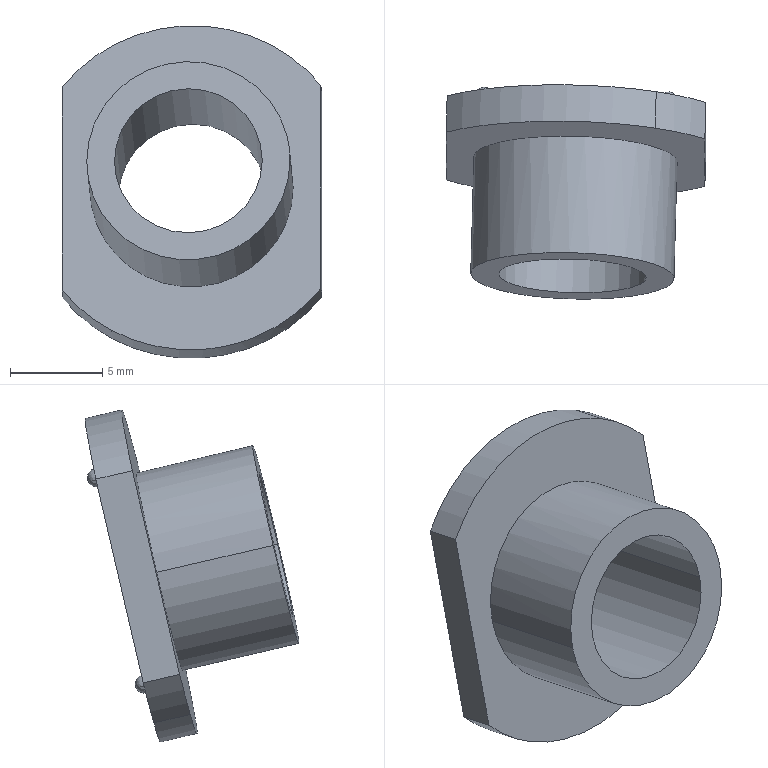Part | STEP file | FNA6101013 | 1 solid | 17 faces | box 14.049 x 11.577 x 17.992 mm | volume 641.835 mm3 | cylinder 8 | plane 5 | sphere 4 | commonest cylinder face diameters 18 x4 8 x2 11 x2
STEP:
#1=CARTESIAN_POINT('',(1542.752,-683.145,923.779));
#2=VERTEX_POINT('',#1);
#3=CARTESIAN_POINT('',(1542.752,-682.919,924.753));
#4=VERTEX_POINT('',#3);
#5=CARTESIAN_POINT('',(1542.752,-683.145,923.779));
#6=CARTESIAN_POINT('',(1542.624,-683.142,923.778));
#7=CARTESIAN_POINT('',(1542.496,-683.129,923.818));
#8=CARTESIAN_POINT('',(1542.386,-683.108,923.897));
#9=CARTESIAN_POINT('',(1542.2,-683.041,924.161));
#10=CARTESIAN_POINT('',(1542.249,-682.965,924.495));
#11=CARTESIAN_POINT('',(1542.38,-682.929,924.667));
#12=CARTESIAN_POINT('',(1542.566,-682.914,924.752));
#13=CARTESIAN_POINT('',(1542.752,-682.919,924.753));
#14=B_SPLINE_CURVE_WITH_KNOTS('',5,(#5,#6,#7,#8,#9,#10,#11,#12,#13),.UNSPECIFIED.,.F.,.U.,(6,3,6),(0.,0.9047,2.221),.UNSPECIFIED.);
#15=EDGE_CURVE('',#2,#4,#14,.T.);
#16=ORIENTED_EDGE('',*,*,#15,.T.);
#17=CARTESIAN_POINT('',(1542.752,-683.145,923.779));
#18=CARTESIAN_POINT('',(1542.88,-683.148,923.78));
#19=CARTESIAN_POINT('',(1543.008,-683.142,923.821));
#20=CARTESIAN_POINT('',(1543.118,-683.126,923.901));
#21=CARTESIAN_POINT('',(1543.305,-683.07,924.167));
#22=CARTESIAN_POINT('',(1543.255,-682.991,924.501));
#23=CARTESIAN_POINT('',(1543.124,-682.948,924.671));
#24=CARTESIAN_POINT('',(1542.938,-682.924,924.754));
#25=CARTESIAN_POINT('',(1542.752,-682.919,924.753));
#26=B_SPLINE_CURVE_WITH_KNOTS('',5,(#17,#18,#19,#20,#21,#22,#23,#24,#25),.UNSPECIFIED.,.F.,.U.,(6,3,6),(0.,0.9047,2.221),.UNSPECIFIED.);
#27=EDGE_CURVE('',#4,#2,#26,.F.);
#28=ORIENTED_EDGE('',*,*,#27,.T.);
#29=EDGE_LOOP('',(#16,#28));
#30=FACE_OUTER_BOUND('',#29,.T.);
#31=CARTESIAN_POINT('',(1542.752,-683.032,924.266));
#32=DIRECTION('',(0.,0.2262,0.9741));
#33=DIRECTION('',(0.9997,-0.02569,0.005964));
#34=AXIS2_PLACEMENT_3D('',#31,#32,#33);
#35=SPHERICAL_SURFACE('',#34,0.5);
#36=ADVANCED_FACE('',(#30),#35,.T.);
#37=CARTESIAN_POINT('',(1530.756,-682.739,924.127));
#38=VERTEX_POINT('',#37);
#39=CARTESIAN_POINT('',(1542.067,-682.523,926.378));
#40=VERTEX_POINT('',#39);
#41=CARTESIAN_POINT('',(1537.754,-684.198,918.659));
#42=DIRECTION('',(0.02637,0.9738,-0.2261));
#43=AXIS2_PLACEMENT_3D('',#41,#42,$);
#44=CIRCLE('',#43,9.);
#45=EDGE_CURVE('',#38,#40,#44,.T.);
#46=ORIENTED_EDGE('',*,*,#45,.T.);
#47=CARTESIAN_POINT('',(1544.751,-683.099,924.211));
#48=VERTEX_POINT('',#47);
#49=CARTESIAN_POINT('',(1537.754,-684.198,918.659));
#50=DIRECTION('',(0.02637,0.9738,-0.2261));
#51=AXIS2_PLACEMENT_3D('',#49,#50,$);
#52=CIRCLE('',#51,9.);
#53=EDGE_CURVE('',#40,#48,#52,.T.);
#54=ORIENTED_EDGE('',*,*,#53,.T.);
#55=CARTESIAN_POINT('',(1544.751,-685.658,913.19));
#56=VERTEX_POINT('',#55);
#57=CARTESIAN_POINT('',(1544.751,-684.378,918.701));
#58=DIRECTION('',(0.,-0.2262,-0.9741));
#59=VECTOR('',#58,1.);
#60=LINE('',#57,#59);
#61=EDGE_CURVE('',#48,#56,#60,.T.);
#62=ORIENTED_EDGE('',*,*,#61,.T.);
#63=CARTESIAN_POINT('',(1533.441,-685.874,910.939));
#64=VERTEX_POINT('',#63);
#65=CARTESIAN_POINT('',(1537.754,-684.198,918.659));
#66=DIRECTION('',(0.02637,0.9738,-0.2261));
#67=AXIS2_PLACEMENT_3D('',#65,#66,$);
#68=CIRCLE('',#67,9.);
#69=EDGE_CURVE('',#56,#64,#68,.T.);
#70=ORIENTED_EDGE('',*,*,#69,.T.);
#71=CARTESIAN_POINT('',(1530.756,-685.298,913.107));
#72=VERTEX_POINT('',#71);
#73=CARTESIAN_POINT('',(1537.754,-684.198,918.659));
#74=DIRECTION('',(0.02637,0.9738,-0.2261));
#75=AXIS2_PLACEMENT_3D('',#73,#74,$);
#76=CIRCLE('',#75,9.);
#77=EDGE_CURVE('',#64,#72,#76,.T.);
#78=ORIENTED_EDGE('',*,*,#77,.T.);
#79=CARTESIAN_POINT('',(1530.756,-684.019,918.617));
#80=DIRECTION('',(0.,0.2262,0.9741));
#81=VECTOR('',#80,1.);
#82=LINE('',#79,#81);
#83=EDGE_CURVE('',#72,#38,#82,.T.);
#84=ORIENTED_EDGE('',*,*,#83,.T.);
#85=EDGE_LOOP('',(#46,#54,#62,#70,#78,#84));
#86=FACE_OUTER_BOUND('',#85,.T.);
#87=CARTESIAN_POINT('',(1532.756,-682.888,923.72));
#88=VERTEX_POINT('',#87);
#89=CARTESIAN_POINT('',(1532.756,-682.662,924.694));
#90=VERTEX_POINT('',#89);
#91=CARTESIAN_POINT('',(1532.756,-682.888,923.72));
#92=CARTESIAN_POINT('',(1532.692,-682.886,923.719));
#93=CARTESIAN_POINT('',(1532.628,-682.882,923.729));
#94=CARTESIAN_POINT('',(1532.567,-682.876,923.748));
#95=CARTESIAN_POINT('',(1532.452,-682.86,923.806));
#96=CARTESIAN_POINT('',(1532.361,-682.837,923.895));
#97=CARTESIAN_POINT('',(1532.324,-682.823,923.947));
#98=CARTESIAN_POINT('',(1532.267,-682.796,924.061));
#99=CARTESIAN_POINT('',(1532.25,-682.766,924.186));
#100=CARTESIAN_POINT('',(1532.252,-682.751,924.25));
#101=CARTESIAN_POINT('',(1532.276,-682.723,924.374));
#102=CARTESIAN_POINT('',(1532.34,-682.699,924.485));
#103=CARTESIAN_POINT('',(1532.381,-682.688,924.535));
#104=CARTESIAN_POINT('',(1532.472,-682.672,924.617));
#105=CARTESIAN_POINT('',(1532.584,-682.663,924.668));
#106=CARTESIAN_POINT('',(1532.64,-682.661,924.685));
#107=CARTESIAN_POINT('',(1532.698,-682.66,924.693));
#108=CARTESIAN_POINT('',(1532.756,-682.662,924.694));
#109=B_SPLINE_CURVE_WITH_KNOTS('',5,(#91,#92,#93,#94,#95,#96,#97,#98,#99,#100,#101,#102,#103,#104,#105,#106,#107,#108),.UNSPECIFIED.,.F.,.U.,(6,3,3,3,3,6),(0.,0.4508,0.9047,1.358,1.812,2.221),.UNSPECIFIED.);
#110=EDGE_CURVE('',#88,#90,#109,.T.);
#111=ORIENTED_EDGE('',*,*,#110,.F.);
#112=CARTESIAN_POINT('',(1532.756,-682.888,923.72));
#113=CARTESIAN_POINT('',(1532.819,-682.89,923.72));
#114=CARTESIAN_POINT('',(1532.883,-682.889,923.73));
#115=CARTESIAN_POINT('',(1532.945,-682.886,923.75));
#116=CARTESIAN_POINT('',(1533.06,-682.875,923.809));
#117=CARTESIAN_POINT('',(1533.15,-682.857,923.9));
#118=CARTESIAN_POINT('',(1533.188,-682.846,923.952));
#119=CARTESIAN_POINT('',(1533.244,-682.821,924.067));
#120=CARTESIAN_POINT('',(1533.261,-682.792,924.192));
#121=CARTESIAN_POINT('',(1533.259,-682.777,924.256));
#122=CARTESIAN_POINT('',(1533.235,-682.748,924.38));
#123=CARTESIAN_POINT('',(1533.171,-682.72,924.49));
#124=CARTESIAN_POINT('',(1533.131,-682.708,924.54));
#125=CARTESIAN_POINT('',(1533.039,-682.687,924.62));
#126=CARTESIAN_POINT('',(1532.928,-682.672,924.67));
#127=CARTESIAN_POINT('',(1532.871,-682.667,924.686));
#128=CARTESIAN_POINT('',(1532.813,-682.663,924.694));
#129=CARTESIAN_POINT('',(1532.756,-682.662,924.694));
#130=B_SPLINE_CURVE_WITH_KNOTS('',5,(#112,#113,#114,#115,#116,#117,#118,#119,#120,#121,#122,#123,#124,#125,#126,#127,#128,#129),.UNSPECIFIED.,.F.,.U.,(6,3,3,3,3,6),(0.,0.4508,0.9047,1.358,1.812,2.221),.UNSPECIFIED.);
#131=EDGE_CURVE('',#90,#88,#130,.F.);
#132=ORIENTED_EDGE('',*,*,#131,.F.);
#133=EDGE_LOOP('',(#111,#132));
#134=FACE_BOUND('',#133,.T.);
#135=ORIENTED_EDGE('',*,*,#15,.F.);
#136=ORIENTED_EDGE('',*,*,#27,.F.);
#137=EDGE_LOOP('',(#135,#136));
#138=FACE_BOUND('',#137,.T.);
#139=CARTESIAN_POINT('',(1542.752,-685.509,913.598));
#140=VERTEX_POINT('',#139);
#141=CARTESIAN_POINT('',(1542.752,-685.735,912.624));
#142=VERTEX_POINT('',#141);
#143=CARTESIAN_POINT('',(1542.752,-685.735,912.624));
#144=CARTESIAN_POINT('',(1542.688,-685.733,912.624));
#145=CARTESIAN_POINT('',(1542.625,-685.729,912.633));
#146=CARTESIAN_POINT('',(1542.563,-685.723,912.653));
#147=CARTESIAN_POINT('',(1542.448,-685.707,912.71));
#148=CARTESIAN_POINT('',(1542.358,-685.683,912.8));
#149=CARTESIAN_POINT('',(1542.32,-685.67,912.852));
#150=CARTESIAN_POINT('',(1542.264,-685.642,912.965));
#151=CARTESIAN_POINT('',(1542.246,-685.613,913.091));
#152=CARTESIAN_POINT('',(1542.248,-685.598,913.154));
#153=CARTESIAN_POINT('',(1542.273,-685.57,913.279));
#154=CARTESIAN_POINT('',(1542.336,-685.546,913.39));
#155=CARTESIAN_POINT('',(1542.377,-685.535,913.44));
#156=CARTESIAN_POINT('',(1542.468,-685.519,913.521));
#157=CARTESIAN_POINT('',(1542.58,-685.51,913.573));
#158=CARTESIAN_POINT('',(1542.636,-685.508,913.589));
#159=CARTESIAN_POINT('',(1542.694,-685.507,913.598));
#160=CARTESIAN_POINT('',(1542.752,-685.509,913.598));
#161=B_SPLINE_CURVE_WITH_KNOTS('',5,(#143,#144,#145,#146,#147,#148,#149,#150,#151,#152,#153,#154,#155,#156,#157,#158,#159,#160),.UNSPECIFIED.,.F.,.U.,(6,3,3,3,3,6),(0.,0.4508,0.9047,1.358,1.812,2.221),.UNSPECIFIED.);
#162=EDGE_CURVE('',#140,#142,#161,.F.);
#163=ORIENTED_EDGE('',*,*,#162,.T.);
#164=CARTESIAN_POINT('',(1542.752,-685.735,912.624));
#165=CARTESIAN_POINT('',(1542.816,-685.737,912.624));
#166=CARTESIAN_POINT('',(1542.88,-685.736,912.635));
#167=CARTESIAN_POINT('',(1542.941,-685.733,912.655));
#168=CARTESIAN_POINT('',(1543.056,-685.722,912.714));
#169=CARTESIAN_POINT('',(1543.147,-685.704,912.805));
#170=CARTESIAN_POINT('',(1543.184,-685.693,912.857));
#171=CARTESIAN_POINT('',(1543.241,-685.668,912.971));
#172=CARTESIAN_POINT('',(1543.258,-685.639,913.097));
#173=CARTESIAN_POINT('',(1543.256,-685.624,913.16));
#174=CARTESIAN_POINT('',(1543.231,-685.595,913.285));
#175=CARTESIAN_POINT('',(1543.168,-685.567,913.395));
#176=CARTESIAN_POINT('',(1543.127,-685.555,913.444));
#177=CARTESIAN_POINT('',(1543.036,-685.533,913.525));
#178=CARTESIAN_POINT('',(1542.924,-685.519,913.575));
#179=CARTESIAN_POINT('',(1542.868,-685.514,913.591));
#180=CARTESIAN_POINT('',(1542.81,-685.51,913.598));
#181=CARTESIAN_POINT('',(1542.752,-685.509,913.598));
#182=B_SPLINE_CURVE_WITH_KNOTS('',5,(#164,#165,#166,#167,#168,#169,#170,#171,#172,#173,#174,#175,#176,#177,#178,#179,#180,#181),.UNSPECIFIED.,.F.,.U.,(6,3,3,3,3,6),(0.,0.4508,0.9047,1.358,1.812,2.221),.UNSPECIFIED.);
#183=EDGE_CURVE('',#142,#140,#182,.T.);
#184=ORIENTED_EDGE('',*,*,#183,.T.);
#185=EDGE_LOOP('',(#163,#184));
#186=FACE_BOUND('',#185,.T.);
#187=CARTESIAN_POINT('',(1532.756,-685.252,913.538));
#188=VERTEX_POINT('',#187);
#189=CARTESIAN_POINT('',(1532.756,-685.478,912.564));
#190=VERTEX_POINT('',#189);
#191=CARTESIAN_POINT('',(1532.756,-685.478,912.564));
#192=CARTESIAN_POINT('',(1532.692,-685.476,912.564));
#193=CARTESIAN_POINT('',(1532.628,-685.472,912.573));
#194=CARTESIAN_POINT('',(1532.567,-685.466,912.593));
#195=CARTESIAN_POINT('',(1532.452,-685.45,912.65));
#196=CARTESIAN_POINT('',(1532.361,-685.427,912.74));
#197=CARTESIAN_POINT('',(1532.324,-685.413,912.792));
#198=CARTESIAN_POINT('',(1532.267,-685.386,912.906));
#199=CARTESIAN_POINT('',(1532.25,-685.356,913.031));
#200=CARTESIAN_POINT('',(1532.252,-685.341,913.095));
#201=CARTESIAN_POINT('',(1532.276,-685.313,913.219));
#202=CARTESIAN_POINT('',(1532.34,-685.289,913.33));
#203=CARTESIAN_POINT('',(1532.381,-685.278,913.38));
#204=CARTESIAN_POINT('',(1532.472,-685.262,913.462));
#205=CARTESIAN_POINT('',(1532.584,-685.253,913.513));
#206=CARTESIAN_POINT('',(1532.64,-685.251,913.53));
#207=CARTESIAN_POINT('',(1532.698,-685.25,913.538));
#208=CARTESIAN_POINT('',(1532.756,-685.252,913.538));
#209=B_SPLINE_CURVE_WITH_KNOTS('',5,(#191,#192,#193,#194,#195,#196,#197,#198,#199,#200,#201,#202,#203,#204,#205,#206,#207,#208),.UNSPECIFIED.,.F.,.U.,(6,3,3,3,3,6),(0.,0.4508,0.9047,1.358,1.812,2.221),.UNSPECIFIED.);
#210=EDGE_CURVE('',#188,#190,#209,.F.);
#211=ORIENTED_EDGE('',*,*,#210,.T.);
#212=CARTESIAN_POINT('',(1532.756,-685.478,912.564));
#213=CARTESIAN_POINT('',(1532.819,-685.48,912.565));
#214=CARTESIAN_POINT('',(1532.883,-685.479,912.575));
#215=CARTESIAN_POINT('',(1532.945,-685.476,912.595));
#216=CARTESIAN_POINT('',(1533.06,-685.465,912.654));
#217=CARTESIAN_POINT('',(1533.15,-685.447,912.745));
#218=CARTESIAN_POINT('',(1533.188,-685.436,912.797));
#219=CARTESIAN_POINT('',(1533.244,-685.411,912.912));
#220=CARTESIAN_POINT('',(1533.261,-685.382,913.037));
#221=CARTESIAN_POINT('',(1533.259,-685.367,913.101));
#222=CARTESIAN_POINT('',(1533.235,-685.338,913.225));
#223=CARTESIAN_POINT('',(1533.171,-685.31,913.335));
#224=CARTESIAN_POINT('',(1533.131,-685.298,913.385));
#225=CARTESIAN_POINT('',(1533.039,-685.277,913.465));
#226=CARTESIAN_POINT('',(1532.928,-685.262,913.515));
#227=CARTESIAN_POINT('',(1532.871,-685.257,913.531));
#228=CARTESIAN_POINT('',(1532.813,-685.253,913.539));
#229=CARTESIAN_POINT('',(1532.756,-685.252,913.538));
#230=B_SPLINE_CURVE_WITH_KNOTS('',5,(#212,#213,#214,#215,#216,#217,#218,#219,#220,#221,#222,#223,#224,#225,#226,#227,#228,#229),.UNSPECIFIED.,.F.,.U.,(6,3,3,3,3,6),(0.,0.4508,0.9047,1.358,1.812,2.221),.UNSPECIFIED.);
#231=EDGE_CURVE('',#190,#188,#230,.T.);
#232=ORIENTED_EDGE('',*,*,#231,.T.);
#233=EDGE_LOOP('',(#211,#232));
#234=FACE_BOUND('',#233,.T.);
#235=CARTESIAN_POINT('',(1541.752,-684.301,918.683));
#236=VERTEX_POINT('',#235);
#237=CARTESIAN_POINT('',(1533.755,-684.096,918.635));
#238=VERTEX_POINT('',#237);
#239=CARTESIAN_POINT('',(1537.754,-684.198,918.659));
#240=DIRECTION('',(0.02637,0.9738,-0.2261));
#241=AXIS2_PLACEMENT_3D('',#239,#240,$);
#242=CIRCLE('',#241,4.);
#243=EDGE_CURVE('',#236,#238,#242,.T.);
#244=ORIENTED_EDGE('',*,*,#243,.F.);
#245=CARTESIAN_POINT('',(1537.754,-684.198,918.659));
#246=DIRECTION('',(0.02637,0.9738,-0.2261));
#247=AXIS2_PLACEMENT_3D('',#245,#246,$);
#248=CIRCLE('',#247,4.);
#249=EDGE_CURVE('',#238,#236,#248,.T.);
#250=ORIENTED_EDGE('',*,*,#249,.F.);
#251=EDGE_LOOP('',(#244,#250));
#252=FACE_BOUND('',#251,.T.);
#253=CARTESIAN_POINT('',(1537.754,-682.672,925.234));
#254=DIRECTION('',(0.02637,0.9738,-0.2261));
#255=DIRECTION('',(0.9997,-0.02569,0.005964));
#256=AXIS2_PLACEMENT_3D('',#253,#254,#255);
#257=PLANE('',#256);
#258=ADVANCED_FACE('',(#86,#134,#138,#186,#234,#252),#257,.T.);
#259=ORIENTED_EDGE('',*,*,#110,.T.);
#260=ORIENTED_EDGE('',*,*,#131,.T.);
#261=EDGE_LOOP('',(#259,#260));
#262=FACE_OUTER_BOUND('',#261,.T.);
#263=CARTESIAN_POINT('',(1532.756,-682.775,924.207));
#264=DIRECTION('',(0.,0.2262,0.9741));
#265=DIRECTION('',(0.9997,-0.02569,0.005964));
#266=AXIS2_PLACEMENT_3D('',#263,#264,#265);
#267=SPHERICAL_SURFACE('',#266,0.5);
#268=ADVANCED_FACE('',(#262),#267,.T.);
#269=CARTESIAN_POINT('',(1543.199,-686.311,919.149));
#270=VERTEX_POINT('',#269);
#271=CARTESIAN_POINT('',(1532.202,-686.029,919.084));
#272=VERTEX_POINT('',#271);
#273=CARTESIAN_POINT('',(1537.7,-686.17,919.117));
#274=DIRECTION('',(-0.02637,-0.9738,0.2261));
#275=AXIS2_PLACEMENT_3D('',#273,#274,$);
#276=CIRCLE('',#275,5.5);
#277=EDGE_CURVE('',#270,#272,#276,.F.);
#278=ORIENTED_EDGE('',*,*,#277,.F.);
#279=CARTESIAN_POINT('',(1543.028,-692.617,920.613));
#280=VERTEX_POINT('',#279);
#281=CARTESIAN_POINT('',(1543.146,-688.247,919.599));
#282=DIRECTION('',(-0.02637,-0.9738,0.2261));
#283=VECTOR('',#282,1.);
#284=LINE('',#281,#283);
#285=EDGE_CURVE('',#280,#270,#284,.F.);
#286=ORIENTED_EDGE('',*,*,#285,.F.);
#287=CARTESIAN_POINT('',(1532.032,-692.334,920.548));
#288=VERTEX_POINT('',#287);
#289=CARTESIAN_POINT('',(1537.53,-692.475,920.581));
#290=DIRECTION('',(-0.02637,-0.9738,0.2261));
#291=AXIS2_PLACEMENT_3D('',#289,#290,$);
#292=CIRCLE('',#291,5.5);
#293=EDGE_CURVE('',#288,#280,#292,.T.);
#294=ORIENTED_EDGE('',*,*,#293,.F.);
#295=CARTESIAN_POINT('',(1532.15,-687.964,919.533));
#296=DIRECTION('',(-0.02637,-0.9738,0.2261));
#297=VECTOR('',#296,1.);
#298=LINE('',#295,#297);
#299=EDGE_CURVE('',#288,#272,#298,.F.);
#300=ORIENTED_EDGE('',*,*,#299,.T.);
#301=EDGE_LOOP('',(#278,#286,#294,#300));
#302=FACE_OUTER_BOUND('',#301,.T.);
#303=CARTESIAN_POINT('',(1537.677,-687.042,919.319));
#304=DIRECTION('',(-0.02637,-0.9738,0.2261));
#305=DIRECTION('',(0.9997,-0.02569,0.005964));
#306=AXIS2_PLACEMENT_3D('',#303,#304,#305);
#307=CYLINDRICAL_SURFACE('',#306,5.5);
#308=ADVANCED_FACE('',(#302),#307,.T.);
#309=CARTESIAN_POINT('',(1533.531,-692.373,920.557));
#310=VERTEX_POINT('',#309);
#311=CARTESIAN_POINT('',(1533.67,-687.26,919.37));
#312=DIRECTION('',(-0.02637,-0.9738,0.2261));
#313=VECTOR('',#312,1.);
#314=LINE('',#311,#313);
#315=EDGE_CURVE('',#310,#238,#314,.F.);
#316=ORIENTED_EDGE('',*,*,#315,.F.);
#317=CARTESIAN_POINT('',(1541.528,-692.578,920.604));
#318=VERTEX_POINT('',#317);
#319=CARTESIAN_POINT('',(1537.53,-692.475,920.581));
#320=DIRECTION('',(-0.02637,-0.9738,0.2261));
#321=AXIS2_PLACEMENT_3D('',#319,#320,$);
#322=CIRCLE('',#321,4.);
#323=EDGE_CURVE('',#310,#318,#322,.T.);
#324=ORIENTED_EDGE('',*,*,#323,.T.);
#325=CARTESIAN_POINT('',(1541.667,-687.466,919.417));
#326=DIRECTION('',(-0.02637,-0.9738,0.2261));
#327=VECTOR('',#326,1.);
#328=LINE('',#325,#327);
#329=EDGE_CURVE('',#318,#236,#328,.F.);
#330=ORIENTED_EDGE('',*,*,#329,.T.);
#331=ORIENTED_EDGE('',*,*,#243,.T.);
#332=EDGE_LOOP('',(#316,#324,#330,#331));
#333=FACE_OUTER_BOUND('',#332,.T.);
#334=CARTESIAN_POINT('',(1537.677,-687.042,919.319));
#335=DIRECTION('',(-0.02637,-0.9738,0.2261));
#336=DIRECTION('',(0.9997,-0.02569,0.005964));
#337=AXIS2_PLACEMENT_3D('',#334,#335,#336);
#338=CYLINDRICAL_SURFACE('',#337,4.);
#339=ADVANCED_FACE('',(#333),#338,.F.);
#340=ORIENTED_EDGE('',*,*,#249,.T.);
#341=ORIENTED_EDGE('',*,*,#329,.F.);
#342=CARTESIAN_POINT('',(1537.53,-692.475,920.581));
#343=DIRECTION('',(-0.02637,-0.9738,0.2261));
#344=AXIS2_PLACEMENT_3D('',#342,#343,$);
#345=CIRCLE('',#344,4.);
#346=EDGE_CURVE('',#318,#310,#345,.T.);
#347=ORIENTED_EDGE('',*,*,#346,.T.);
#348=ORIENTED_EDGE('',*,*,#315,.T.);
#349=EDGE_LOOP('',(#340,#341,#347,#348));
#350=FACE_OUTER_BOUND('',#349,.T.);
#351=ADVANCED_FACE('',(#350),#338,.F.);
#352=CARTESIAN_POINT('',(1532.032,-692.334,920.548));
#353=CARTESIAN_POINT('',(1532.032,-692.139,921.389));
#354=CARTESIAN_POINT('',(1532.201,-691.948,922.232));
#355=CARTESIAN_POINT('',(1532.541,-691.771,923.032));
#356=CARTESIAN_POINT('',(1533.522,-691.466,924.462));
#357=CARTESIAN_POINT('',(1534.983,-691.281,925.427));
#358=CARTESIAN_POINT('',(1535.802,-691.225,925.762));
#359=CARTESIAN_POINT('',(1537.53,-691.193,926.103));
#360=CARTESIAN_POINT('',(1539.257,-691.314,925.783));
#361=CARTESIAN_POINT('',(1540.076,-691.412,925.457));
#362=CARTESIAN_POINT('',(1541.537,-691.672,924.51));
#363=CARTESIAN_POINT('',(1542.519,-692.027,923.092));
#364=CARTESIAN_POINT('',(1542.858,-692.221,922.295));
#365=CARTESIAN_POINT('',(1543.028,-692.421,921.455));
#366=CARTESIAN_POINT('',(1543.028,-692.617,920.613));
#367=B_SPLINE_CURVE_WITH_KNOTS('',5,(#352,#353,#354,#355,#356,#357,#358,#359,#360,#361,#362,#363,#364,#365,#366),.UNSPECIFIED.,.F.,.U.,(6,3,3,3,6),(53.08,61.72,70.359,78.998,87.638),.UNSPECIFIED.);
#368=EDGE_CURVE('',#280,#288,#367,.F.);
#369=ORIENTED_EDGE('',*,*,#368,.T.);
#370=ORIENTED_EDGE('',*,*,#293,.T.);
#371=EDGE_LOOP('',(#369,#370));
#372=FACE_OUTER_BOUND('',#371,.T.);
#373=ORIENTED_EDGE('',*,*,#346,.F.);
#374=ORIENTED_EDGE('',*,*,#323,.F.);
#375=EDGE_LOOP('',(#373,#374));
#376=FACE_BOUND('',#375,.T.);
#377=CARTESIAN_POINT('',(1537.53,-692.475,920.581));
#378=DIRECTION('',(0.02637,0.9738,-0.2261));
#379=DIRECTION('',(-0.0564,0.1138,0.4836));
#380=AXIS2_PLACEMENT_3D('',#377,#378,#379);
#381=PLANE('',#380);
#382=ADVANCED_FACE('',(#372,#376),#381,.F.);
#383=ORIENTED_EDGE('',*,*,#299,.F.);
#384=ORIENTED_EDGE('',*,*,#368,.F.);
#385=ORIENTED_EDGE('',*,*,#285,.T.);
#386=CARTESIAN_POINT('',(1537.7,-686.17,919.117));
#387=DIRECTION('',(-0.02637,-0.9738,0.2261));
#388=AXIS2_PLACEMENT_3D('',#386,#387,$);
#389=CIRCLE('',#388,5.5);
#390=EDGE_CURVE('',#272,#270,#389,.F.);
#391=ORIENTED_EDGE('',*,*,#390,.F.);
#392=EDGE_LOOP('',(#383,#384,#385,#391));
#393=FACE_OUTER_BOUND('',#392,.T.);
#394=ADVANCED_FACE('',(#393),#307,.T.);
#395=ORIENTED_EDGE('',*,*,#53,.F.);
#396=CARTESIAN_POINT('',(1542.014,-684.495,926.836));
#397=VERTEX_POINT('',#396);
#398=CARTESIAN_POINT('',(1542.041,-683.509,926.607));
#399=DIRECTION('',(0.02637,0.9738,-0.2261));
#400=VECTOR('',#399,1.);
#401=LINE('',#398,#400);
#402=EDGE_CURVE('',#397,#40,#401,.T.);
#403=ORIENTED_EDGE('',*,*,#402,.F.);
#404=CARTESIAN_POINT('',(1544.698,-685.071,924.669));
#405=VERTEX_POINT('',#404);
#406=CARTESIAN_POINT('',(1537.7,-686.17,919.117));
#407=DIRECTION('',(0.02637,0.9738,-0.2261));
#408=AXIS2_PLACEMENT_3D('',#406,#407,$);
#409=CIRCLE('',#408,9.);
#410=EDGE_CURVE('',#405,#397,#409,.F.);
#411=ORIENTED_EDGE('',*,*,#410,.F.);
#412=CARTESIAN_POINT('',(1544.725,-684.085,924.44));
#413=DIRECTION('',(0.02637,0.9738,-0.2261));
#414=VECTOR('',#413,1.);
#415=LINE('',#412,#414);
#416=EDGE_CURVE('',#48,#405,#415,.F.);
#417=ORIENTED_EDGE('',*,*,#416,.F.);
#418=EDGE_LOOP('',(#395,#403,#411,#417));
#419=FACE_OUTER_BOUND('',#418,.T.);
#420=CARTESIAN_POINT('',(1537.668,-687.363,919.394));
#421=DIRECTION('',(0.02637,0.9738,-0.2261));
#422=DIRECTION('',(0.4793,0.1862,0.8577));
#423=AXIS2_PLACEMENT_3D('',#420,#421,#422);
#424=CYLINDRICAL_SURFACE('',#423,9.);
#425=ADVANCED_FACE('',(#419),#424,.T.);
#426=ORIENTED_EDGE('',*,*,#45,.F.);
#427=CARTESIAN_POINT('',(1530.703,-684.711,924.585));
#428=VERTEX_POINT('',#427);
#429=CARTESIAN_POINT('',(1530.73,-683.725,924.356));
#430=DIRECTION('',(0.02637,0.9738,-0.2261));
#431=VECTOR('',#430,1.);
#432=LINE('',#429,#431);
#433=EDGE_CURVE('',#38,#428,#432,.F.);
#434=ORIENTED_EDGE('',*,*,#433,.T.);
#435=CARTESIAN_POINT('',(1537.7,-686.17,919.117));
#436=DIRECTION('',(0.02637,0.9738,-0.2261));
#437=AXIS2_PLACEMENT_3D('',#435,#436,$);
#438=CIRCLE('',#437,9.);
#439=EDGE_CURVE('',#397,#428,#438,.F.);
#440=ORIENTED_EDGE('',*,*,#439,.F.);
#441=ORIENTED_EDGE('',*,*,#402,.T.);
#442=EDGE_LOOP('',(#426,#434,#440,#441));
#443=FACE_OUTER_BOUND('',#442,.T.);
#444=ADVANCED_FACE('',(#443),#424,.T.);
#445=CARTESIAN_POINT('',(1533.387,-687.846,911.397));
#446=VERTEX_POINT('',#445);
#447=CARTESIAN_POINT('',(1544.698,-687.629,913.648));
#448=VERTEX_POINT('',#447);
#449=CARTESIAN_POINT('',(1533.387,-687.846,911.397));
#450=CARTESIAN_POINT('',(1535.584,-688.174,910.241));
#451=CARTESIAN_POINT('',(1538.198,-688.34,909.83));
#452=CARTESIAN_POINT('',(1540.875,-688.289,910.362));
#453=CARTESIAN_POINT('',(1543.125,-688.029,911.742));
#454=CARTESIAN_POINT('',(1544.698,-687.629,913.648));
#455=B_SPLINE_CURVE_WITH_KNOTS('',5,(#449,#450,#451,#452,#453,#454),.UNSPECIFIED.,.F.,.U.,(6,6),(47.549,72.589),.UNSPECIFIED.);
#456=EDGE_CURVE('',#446,#448,#455,.T.);
#457=ORIENTED_EDGE('',*,*,#456,.T.);
#458=CARTESIAN_POINT('',(1544.698,-686.88,916.874));
#459=VERTEX_POINT('',#458);
#460=CARTESIAN_POINT('',(1544.698,-687.629,913.648));
#461=CARTESIAN_POINT('',(1544.698,-686.88,916.874));
#462=B_SPLINE_CURVE_WITH_KNOTS('',1,(#460,#461),.UNSPECIFIED.,.F.,.U.,(2,2),(-11.314,-4.69),.UNSPECIFIED.);
#463=EDGE_CURVE('',#448,#459,#462,.T.);
#464=ORIENTED_EDGE('',*,*,#463,.T.);
#465=CARTESIAN_POINT('',(1544.698,-685.82,921.443));
#466=VERTEX_POINT('',#465);
#467=CARTESIAN_POINT('',(1544.698,-686.88,916.874));
#468=CARTESIAN_POINT('',(1544.698,-685.82,921.443));
#469=B_SPLINE_CURVE_WITH_KNOTS('',1,(#467,#468),.UNSPECIFIED.,.F.,.U.,(2,2),(-4.69,4.69),.UNSPECIFIED.);
#470=EDGE_CURVE('',#459,#466,#469,.T.);
#471=ORIENTED_EDGE('',*,*,#470,.T.);
#472=CARTESIAN_POINT('',(1544.698,-685.82,921.443));
#473=CARTESIAN_POINT('',(1544.698,-685.071,924.669));
#474=B_SPLINE_CURVE_WITH_KNOTS('',1,(#472,#473),.UNSPECIFIED.,.F.,.U.,(2,2),(4.69,11.314),.UNSPECIFIED.);
#475=EDGE_CURVE('',#466,#405,#474,.T.);
#476=ORIENTED_EDGE('',*,*,#475,.T.);
#477=ORIENTED_EDGE('',*,*,#410,.T.);
#478=ORIENTED_EDGE('',*,*,#439,.T.);
#479=CARTESIAN_POINT('',(1530.703,-685.46,921.359));
#480=VERTEX_POINT('',#479);
#481=CARTESIAN_POINT('',(1530.703,-685.46,921.359));
#482=CARTESIAN_POINT('',(1530.703,-684.711,924.585));
#483=B_SPLINE_CURVE_WITH_KNOTS('',1,(#481,#482),.UNSPECIFIED.,.F.,.U.,(2,2),(4.69,11.314),.UNSPECIFIED.);
#484=EDGE_CURVE('',#480,#428,#483,.T.);
#485=ORIENTED_EDGE('',*,*,#484,.F.);
#486=CARTESIAN_POINT('',(1530.703,-686.521,916.79));
#487=VERTEX_POINT('',#486);
#488=CARTESIAN_POINT('',(1530.703,-686.521,916.79));
#489=CARTESIAN_POINT('',(1530.703,-685.46,921.359));
#490=B_SPLINE_CURVE_WITH_KNOTS('',1,(#488,#489),.UNSPECIFIED.,.F.,.U.,(2,2),(-4.69,4.69),.UNSPECIFIED.);
#491=EDGE_CURVE('',#487,#480,#490,.T.);
#492=ORIENTED_EDGE('',*,*,#491,.F.);
#493=CARTESIAN_POINT('',(1530.703,-687.27,913.565));
#494=VERTEX_POINT('',#493);
#495=CARTESIAN_POINT('',(1530.703,-687.27,913.565));
#496=CARTESIAN_POINT('',(1530.703,-686.521,916.79));
#497=B_SPLINE_CURVE_WITH_KNOTS('',1,(#495,#496),.UNSPECIFIED.,.F.,.U.,(2,2),(-11.314,-4.69),.UNSPECIFIED.);
#498=EDGE_CURVE('',#494,#487,#497,.T.);
#499=ORIENTED_EDGE('',*,*,#498,.F.);
#500=CARTESIAN_POINT('',(1530.703,-687.27,913.565));
#501=CARTESIAN_POINT('',(1531.44,-687.495,912.68));
#502=CARTESIAN_POINT('',(1532.358,-687.692,911.939));
#503=CARTESIAN_POINT('',(1533.387,-687.846,911.397));
#504=B_SPLINE_CURVE_WITH_KNOTS('',3,(#500,#501,#502,#503),.UNSPECIFIED.,.F.,.U.,(4,4),(40.508,47.549),.UNSPECIFIED.);
#505=EDGE_CURVE('',#494,#446,#504,.T.);
#506=ORIENTED_EDGE('',*,*,#505,.T.);
#507=EDGE_LOOP('',(#457,#464,#471,#476,#477,#478,#485,#492,#499,#506));
#508=FACE_OUTER_BOUND('',#507,.T.);
#509=ORIENTED_EDGE('',*,*,#390,.T.);
#510=ORIENTED_EDGE('',*,*,#277,.T.);
#511=EDGE_LOOP('',(#509,#510));
#512=FACE_BOUND('',#511,.T.);
#513=CARTESIAN_POINT('',(1537.7,-686.17,919.117));
#514=DIRECTION('',(-0.02637,-0.9738,0.2261));
#515=DIRECTION('',(0.000000609,0.1131,0.487));
#516=AXIS2_PLACEMENT_3D('',#513,#514,#515);
#517=PLANE('',#516);
#518=ADVANCED_FACE('',(#508,#512),#517,.T.);
#519=ORIENTED_EDGE('',*,*,#416,.T.);
#520=ORIENTED_EDGE('',*,*,#475,.F.);
#521=ORIENTED_EDGE('',*,*,#470,.F.);
#522=ORIENTED_EDGE('',*,*,#463,.F.);
#523=CARTESIAN_POINT('',(1544.725,-686.643,913.419));
#524=DIRECTION('',(0.02637,0.9738,-0.2261));
#525=VECTOR('',#524,1.);
#526=LINE('',#523,#525);
#527=EDGE_CURVE('',#56,#448,#526,.F.);
#528=ORIENTED_EDGE('',*,*,#527,.F.);
#529=ORIENTED_EDGE('',*,*,#61,.F.);
#530=EDGE_LOOP('',(#519,#520,#521,#522,#528,#529));
#531=FACE_OUTER_BOUND('',#530,.T.);
#532=CARTESIAN_POINT('',(1544.845,-680.914,917.896));
#533=DIRECTION('',(0.9997,-0.02569,0.005964));
#534=DIRECTION('',(0.01318,0.4869,-0.113));
#535=AXIS2_PLACEMENT_3D('',#532,#533,#534);
#536=PLANE('',#535);
#537=ADVANCED_FACE('',(#531),#536,.T.);
#538=CARTESIAN_POINT('',(1533.414,-686.86,911.168));
#539=DIRECTION('',(0.02637,0.9738,-0.2261));
#540=VECTOR('',#539,1.);
#541=LINE('',#538,#540);
#542=EDGE_CURVE('',#446,#64,#541,.T.);
#543=ORIENTED_EDGE('',*,*,#542,.T.);
#544=ORIENTED_EDGE('',*,*,#69,.F.);
#545=ORIENTED_EDGE('',*,*,#527,.T.);
#546=ORIENTED_EDGE('',*,*,#456,.F.);
#547=EDGE_LOOP('',(#543,#544,#545,#546));
#548=FACE_OUTER_BOUND('',#547,.T.);
#549=CARTESIAN_POINT('',(1537.668,-687.363,919.394));
#550=DIRECTION('',(0.02637,0.9738,-0.2261));
#551=DIRECTION('',(0.4793,0.1862,0.8577));
#552=AXIS2_PLACEMENT_3D('',#549,#550,#551);
#553=CYLINDRICAL_SURFACE('',#552,9.);
#554=ADVANCED_FACE('',(#548),#553,.T.);
#555=ORIENTED_EDGE('',*,*,#505,.F.);
#556=CARTESIAN_POINT('',(1530.73,-686.284,913.336));
#557=DIRECTION('',(0.02637,0.9738,-0.2261));
#558=VECTOR('',#557,1.);
#559=LINE('',#556,#558);
#560=EDGE_CURVE('',#72,#494,#559,.F.);
#561=ORIENTED_EDGE('',*,*,#560,.F.);
#562=ORIENTED_EDGE('',*,*,#77,.F.);
#563=ORIENTED_EDGE('',*,*,#542,.F.);
#564=EDGE_LOOP('',(#555,#561,#562,#563));
#565=FACE_OUTER_BOUND('',#564,.T.);
#566=ADVANCED_FACE('',(#565),#553,.T.);
#567=ORIENTED_EDGE('',*,*,#433,.F.);
#568=ORIENTED_EDGE('',*,*,#83,.F.);
#569=ORIENTED_EDGE('',*,*,#560,.T.);
#570=ORIENTED_EDGE('',*,*,#498,.T.);
#571=ORIENTED_EDGE('',*,*,#491,.T.);
#572=ORIENTED_EDGE('',*,*,#484,.T.);
#573=EDGE_LOOP('',(#567,#568,#569,#570,#571,#572));
#574=FACE_OUTER_BOUND('',#573,.T.);
#575=CARTESIAN_POINT('',(1530.85,-680.555,917.813));
#576=DIRECTION('',(0.9997,-0.02569,0.005964));
#577=DIRECTION('',(0.01318,0.4869,-0.113));
#578=AXIS2_PLACEMENT_3D('',#575,#576,#577);
#579=PLANE('',#578);
#580=ADVANCED_FACE('',(#574),#579,.F.);
#581=ORIENTED_EDGE('',*,*,#183,.F.);
#582=ORIENTED_EDGE('',*,*,#162,.F.);
#583=EDGE_LOOP('',(#581,#582));
#584=FACE_OUTER_BOUND('',#583,.T.);
#585=CARTESIAN_POINT('',(1542.752,-685.622,913.111));
#586=DIRECTION('',(0.,0.2262,0.9741));
#587=DIRECTION('',(0.9997,-0.02569,0.005964));
#588=AXIS2_PLACEMENT_3D('',#585,#586,#587);
#589=SPHERICAL_SURFACE('',#588,0.5);
#590=ADVANCED_FACE('',(#584),#589,.T.);
#591=ORIENTED_EDGE('',*,*,#231,.F.);
#592=ORIENTED_EDGE('',*,*,#210,.F.);
#593=EDGE_LOOP('',(#591,#592));
#594=FACE_OUTER_BOUND('',#593,.T.);
#595=CARTESIAN_POINT('',(1532.756,-685.365,913.051));
#596=DIRECTION('',(0.,0.2262,0.9741));
#597=DIRECTION('',(0.9997,-0.02569,0.005964));
#598=AXIS2_PLACEMENT_3D('',#595,#596,#597);
#599=SPHERICAL_SURFACE('',#598,0.5);
#600=ADVANCED_FACE('',(#594),#599,.T.);
#601=CLOSED_SHELL('',(#36,#258,#268,#308,#339,#351,#382,#394,#425,#444,#518,#537,#554,#566,#580,#590,#600));
#602=MANIFOLD_SOLID_BREP('',#601);
#603=(LENGTH_UNIT()NAMED_UNIT(*)SI_UNIT(.MILLI.,.METRE.));
#604=UNCERTAINTY_MEASURE_WITH_UNIT(LENGTH_MEASURE(0.005),#603,'','');
#605=(NAMED_UNIT(*)PLANE_ANGLE_UNIT()SI_UNIT($,.RADIAN.));
#606=(NAMED_UNIT(*)SI_UNIT($,.STERADIAN.)SOLID_ANGLE_UNIT());
#607=(GEOMETRIC_REPRESENTATION_CONTEXT(3)GLOBAL_UNCERTAINTY_ASSIGNED_CONTEXT((#604))GLOBAL_UNIT_ASSIGNED_CONTEXT((#603,#605,#606))REPRESENTATION_CONTEXT('',''));
#608=ADVANCED_BREP_SHAPE_REPRESENTATION('',(#602),#607);